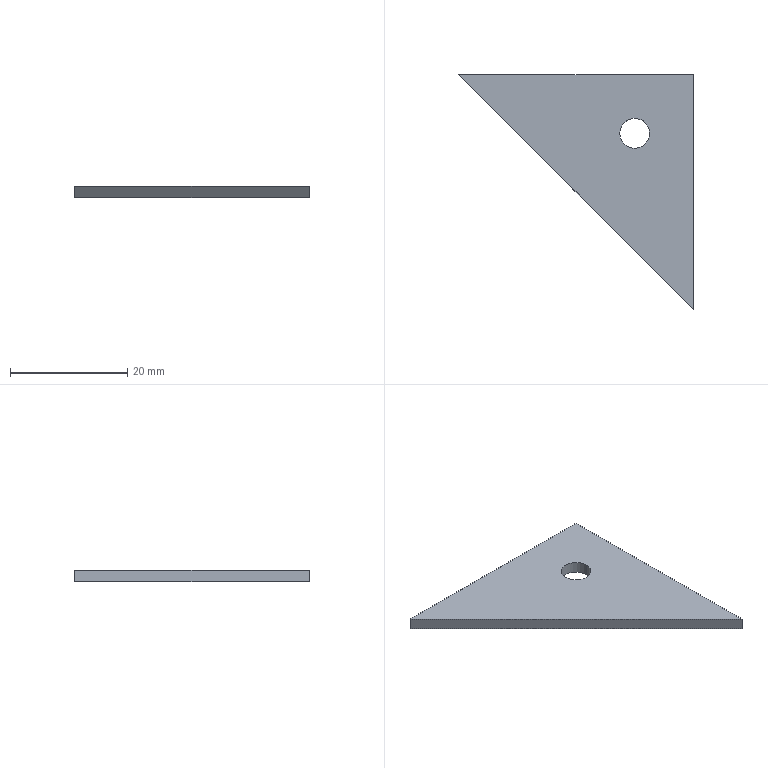Part | SolidWorks | features FlatPattern 1, SMBaseFlange 1, SheetMetal 1 | 1 solid | 7 faces | box 40 x 40 x 2 mm | volume 1559 mm3 | plane 5 | cylinder 2 | commonest cylinder face diameters 5.1 x2
STEP:
#1=CARTESIAN_POINT('',(7.45,10.,-2.));
#2=VERTEX_POINT('',#1);
#3=CARTESIAN_POINT('',(12.55,10.,-2.));
#4=VERTEX_POINT('',#3);
#5=CARTESIAN_POINT('',(10.,10.,-2.));
#6=DIRECTION('',(0.,0.,1.));
#7=DIRECTION('',(1.,0.,0.));
#8=AXIS2_PLACEMENT_3D('',#5,#6,#7);
#9=CIRCLE('',#8,2.55);
#10=EDGE_CURVE('',#2,#4,#9,.T.);
#11=ORIENTED_EDGE('',*,*,#10,.F.);
#12=CARTESIAN_POINT('',(7.45,10.,0.));
#13=VERTEX_POINT('',#12);
#14=CARTESIAN_POINT('',(7.45,10.,-2.));
#15=DIRECTION('',(0.,0.,1.));
#16=VECTOR('',#15,1000.);
#17=LINE('',#14,#16);
#18=EDGE_CURVE('',#2,#13,#17,.T.);
#19=ORIENTED_EDGE('',*,*,#18,.T.);
#20=CARTESIAN_POINT('',(12.55,10.,0.));
#21=VERTEX_POINT('',#20);
#22=CARTESIAN_POINT('',(10.,10.,0.));
#23=DIRECTION('',(0.,0.,1.));
#24=DIRECTION('',(1.,0.,0.));
#25=AXIS2_PLACEMENT_3D('',#22,#23,#24);
#26=CIRCLE('',#25,2.55);
#27=EDGE_CURVE('',#13,#21,#26,.T.);
#28=ORIENTED_EDGE('',*,*,#27,.T.);
#29=CARTESIAN_POINT('',(12.55,10.,-2.));
#30=DIRECTION('',(0.,0.,1.));
#31=VECTOR('',#30,1000.);
#32=LINE('',#29,#31);
#33=EDGE_CURVE('',#4,#21,#32,.T.);
#34=ORIENTED_EDGE('',*,*,#33,.F.);
#35=EDGE_LOOP('',(#11,#19,#28,#34));
#36=FACE_OUTER_BOUND('',#35,.T.);
#37=CARTESIAN_POINT('',(10.,10.,-2.));
#38=DIRECTION('',(0.,0.,1.));
#39=DIRECTION('',(1.,0.,0.));
#40=AXIS2_PLACEMENT_3D('',#37,#38,#39);
#41=CYLINDRICAL_SURFACE('',#40,2.55);
#42=ADVANCED_FACE('',(#36),#41,.F.);
#43=CARTESIAN_POINT('',(20.,-20.,0.));
#44=VERTEX_POINT('',#43);
#45=CARTESIAN_POINT('',(20.,20.,0.));
#46=VERTEX_POINT('',#45);
#47=CARTESIAN_POINT('',(20.,20.,0.));
#48=DIRECTION('',(0.,1.,0.));
#49=VECTOR('',#48,1000.);
#50=LINE('',#47,#49);
#51=EDGE_CURVE('',#44,#46,#50,.T.);
#52=ORIENTED_EDGE('',*,*,#51,.F.);
#53=CARTESIAN_POINT('',(20.,-20.,-2.));
#54=VERTEX_POINT('',#53);
#55=CARTESIAN_POINT('',(20.,-20.,-2.));
#56=DIRECTION('',(0.,0.,1.));
#57=VECTOR('',#56,1000.);
#58=LINE('',#55,#57);
#59=EDGE_CURVE('',#54,#44,#58,.T.);
#60=ORIENTED_EDGE('',*,*,#59,.F.);
#61=CARTESIAN_POINT('',(20.,20.,-2.));
#62=VERTEX_POINT('',#61);
#63=CARTESIAN_POINT('',(20.,20.,-2.));
#64=DIRECTION('',(0.,1.,0.));
#65=VECTOR('',#64,1000.);
#66=LINE('',#63,#65);
#67=EDGE_CURVE('',#54,#62,#66,.T.);
#68=ORIENTED_EDGE('',*,*,#67,.T.);
#69=CARTESIAN_POINT('',(20.,20.,-2.));
#70=DIRECTION('',(0.,0.,1.));
#71=VECTOR('',#70,1000.);
#72=LINE('',#69,#71);
#73=EDGE_CURVE('',#62,#46,#72,.T.);
#74=ORIENTED_EDGE('',*,*,#73,.T.);
#75=EDGE_LOOP('',(#52,#60,#68,#74));
#76=FACE_OUTER_BOUND('',#75,.T.);
#77=CARTESIAN_POINT('',(20.,20.,-2.));
#78=DIRECTION('',(1.,0.,0.));
#79=DIRECTION('',(0.,1.,0.));
#80=AXIS2_PLACEMENT_3D('',#77,#78,#79);
#81=PLANE('',#80);
#82=ADVANCED_FACE('',(#76),#81,.T.);
#83=CARTESIAN_POINT('',(-20.,20.,0.));
#84=VERTEX_POINT('',#83);
#85=CARTESIAN_POINT('',(-20.,20.,0.));
#86=DIRECTION('',(0.7071,-0.7071,0.));
#87=VECTOR('',#86,1000.);
#88=LINE('',#85,#87);
#89=EDGE_CURVE('',#84,#44,#88,.T.);
#90=ORIENTED_EDGE('',*,*,#89,.F.);
#91=CARTESIAN_POINT('',(-20.,20.,-2.));
#92=VERTEX_POINT('',#91);
#93=CARTESIAN_POINT('',(-20.,20.,-2.));
#94=DIRECTION('',(0.,0.,1.));
#95=VECTOR('',#94,1000.);
#96=LINE('',#93,#95);
#97=EDGE_CURVE('',#92,#84,#96,.T.);
#98=ORIENTED_EDGE('',*,*,#97,.F.);
#99=CARTESIAN_POINT('',(-20.,20.,-2.));
#100=DIRECTION('',(0.7071,-0.7071,0.));
#101=VECTOR('',#100,1000.);
#102=LINE('',#99,#101);
#103=EDGE_CURVE('',#92,#54,#102,.T.);
#104=ORIENTED_EDGE('',*,*,#103,.T.);
#105=ORIENTED_EDGE('',*,*,#59,.T.);
#106=EDGE_LOOP('',(#90,#98,#104,#105));
#107=FACE_OUTER_BOUND('',#106,.T.);
#108=CARTESIAN_POINT('',(-20.,20.,-2.));
#109=DIRECTION('',(-0.7071,-0.7071,0.));
#110=DIRECTION('',(0.7071,-0.7071,0.));
#111=AXIS2_PLACEMENT_3D('',#108,#109,#110);
#112=PLANE('',#111);
#113=ADVANCED_FACE('',(#107),#112,.T.);
#114=CARTESIAN_POINT('',(-20.,20.,0.));
#115=DIRECTION('',(-1.,0.,0.));
#116=VECTOR('',#115,1000.);
#117=LINE('',#114,#116);
#118=EDGE_CURVE('',#46,#84,#117,.T.);
#119=ORIENTED_EDGE('',*,*,#118,.F.);
#120=ORIENTED_EDGE('',*,*,#73,.F.);
#121=CARTESIAN_POINT('',(-20.,20.,-2.));
#122=DIRECTION('',(-1.,0.,0.));
#123=VECTOR('',#122,1000.);
#124=LINE('',#121,#123);
#125=EDGE_CURVE('',#62,#92,#124,.T.);
#126=ORIENTED_EDGE('',*,*,#125,.T.);
#127=ORIENTED_EDGE('',*,*,#97,.T.);
#128=EDGE_LOOP('',(#119,#120,#126,#127));
#129=FACE_OUTER_BOUND('',#128,.T.);
#130=CARTESIAN_POINT('',(-20.,20.,-2.));
#131=DIRECTION('',(0.,1.,0.));
#132=DIRECTION('',(0.,0.,1.));
#133=AXIS2_PLACEMENT_3D('',#130,#131,#132);
#134=PLANE('',#133);
#135=ADVANCED_FACE('',(#129),#134,.T.);
#136=CARTESIAN_POINT('',(10.,10.,-2.));
#137=DIRECTION('',(0.,0.,1.));
#138=DIRECTION('',(1.,0.,0.));
#139=AXIS2_PLACEMENT_3D('',#136,#137,#138);
#140=CIRCLE('',#139,2.55);
#141=EDGE_CURVE('',#4,#2,#140,.T.);
#142=ORIENTED_EDGE('',*,*,#141,.T.);
#143=ORIENTED_EDGE('',*,*,#10,.T.);
#144=EDGE_LOOP('',(#142,#143));
#145=FACE_BOUND('',#144,.T.);
#146=ORIENTED_EDGE('',*,*,#67,.F.);
#147=ORIENTED_EDGE('',*,*,#103,.F.);
#148=ORIENTED_EDGE('',*,*,#125,.F.);
#149=EDGE_LOOP('',(#146,#147,#148));
#150=FACE_OUTER_BOUND('',#149,.T.);
#151=CARTESIAN_POINT('',(0.,0.,-2.));
#152=DIRECTION('',(0.,0.,1.));
#153=DIRECTION('',(1.,0.,0.));
#154=AXIS2_PLACEMENT_3D('',#151,#152,#153);
#155=PLANE('',#154);
#156=ADVANCED_FACE('',(#145,#150),#155,.F.);
#157=CARTESIAN_POINT('',(10.,10.,0.));
#158=DIRECTION('',(0.,0.,1.));
#159=DIRECTION('',(1.,0.,0.));
#160=AXIS2_PLACEMENT_3D('',#157,#158,#159);
#161=CIRCLE('',#160,2.55);
#162=EDGE_CURVE('',#21,#13,#161,.T.);
#163=ORIENTED_EDGE('',*,*,#162,.F.);
#164=ORIENTED_EDGE('',*,*,#27,.F.);
#165=EDGE_LOOP('',(#163,#164));
#166=FACE_BOUND('',#165,.T.);
#167=ORIENTED_EDGE('',*,*,#51,.T.);
#168=ORIENTED_EDGE('',*,*,#118,.T.);
#169=ORIENTED_EDGE('',*,*,#89,.T.);
#170=EDGE_LOOP('',(#167,#168,#169));
#171=FACE_OUTER_BOUND('',#170,.T.);
#172=CARTESIAN_POINT('',(0.,0.,0.));
#173=DIRECTION('',(0.,0.,1.));
#174=DIRECTION('',(1.,0.,0.));
#175=AXIS2_PLACEMENT_3D('',#172,#173,#174);
#176=PLANE('',#175);
#177=ADVANCED_FACE('',(#166,#171),#176,.T.);
#178=ORIENTED_EDGE('',*,*,#18,.F.);
#179=ORIENTED_EDGE('',*,*,#141,.F.);
#180=ORIENTED_EDGE('',*,*,#33,.T.);
#181=ORIENTED_EDGE('',*,*,#162,.T.);
#182=EDGE_LOOP('',(#178,#179,#180,#181));
#183=FACE_OUTER_BOUND('',#182,.T.);
#184=CARTESIAN_POINT('',(10.,10.,-2.));
#185=DIRECTION('',(0.,0.,1.));
#186=DIRECTION('',(1.,0.,0.));
#187=AXIS2_PLACEMENT_3D('',#184,#185,#186);
#188=CYLINDRICAL_SURFACE('',#187,2.55);
#189=ADVANCED_FACE('',(#183),#188,.F.);
#190=CLOSED_SHELL('',(#42,#82,#113,#135,#156,#177,#189));
#191=MANIFOLD_SOLID_BREP('',#190);
#192=CARTESIAN_POINT('',(0.,0.,0.));
#193=DIRECTION('',(0.,0.,1.));
#194=DIRECTION('',(1.,0.,0.));
#195=AXIS2_PLACEMENT_3D('',#192,#193,#194);
#196=(LENGTH_UNIT()NAMED_UNIT(*)SI_UNIT(.MILLI.,.METRE.));
#197=UNCERTAINTY_MEASURE_WITH_UNIT(LENGTH_MEASURE(0.00001),#196,'','');
#198=(NAMED_UNIT(*)PLANE_ANGLE_UNIT()SI_UNIT($,.RADIAN.));
#199=(NAMED_UNIT(*)SI_UNIT($,.STERADIAN.)SOLID_ANGLE_UNIT());
#200=(GEOMETRIC_REPRESENTATION_CONTEXT(3)GLOBAL_UNCERTAINTY_ASSIGNED_CONTEXT((#197))GLOBAL_UNIT_ASSIGNED_CONTEXT((#196,#198,#199))REPRESENTATION_CONTEXT('',''));
#201=ADVANCED_BREP_SHAPE_REPRESENTATION('',(#191,#195),#200);